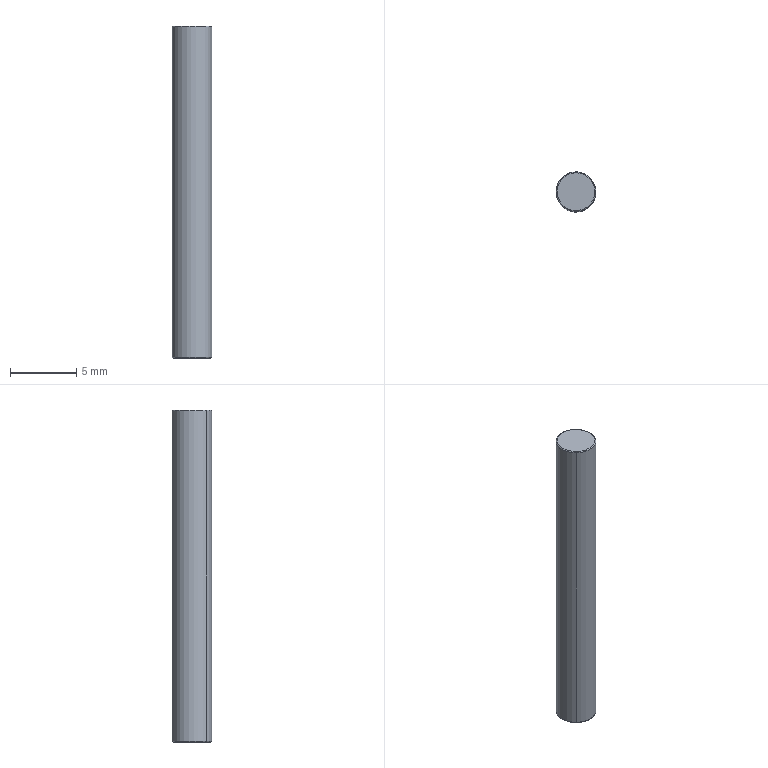Part | SolidWorks | features SplitBody 1 | 1 solid | 8 faces | box 3 x 3 x 25 mm | volume 176.692 mm3 | torus 4 | cylinder 2 | plane 2 | commonest cylinder face diameters 3 x2
STEP:
#1=CARTESIAN_POINT('',(423.091,-5.089,-249.647));
#2=VERTEX_POINT('',#1);
#3=CARTESIAN_POINT('',(425.059,-3.028,-249.647));
#4=VERTEX_POINT('',#3);
#5=CARTESIAN_POINT('',(424.075,-4.058,-249.647));
#6=DIRECTION('',(0.,0.,1.));
#7=DIRECTION('',(0.6906,0.7232,0.));
#8=AXIS2_PLACEMENT_3D('',#5,#6,#7);
#9=CIRCLE('',#8,1.425);
#10=EDGE_CURVE('',#2,#4,#9,.T.);
#11=ORIENTED_EDGE('',*,*,#10,.F.);
#12=CARTESIAN_POINT('',(423.039,-5.143,-249.722));
#13=VERTEX_POINT('',#12);
#14=CARTESIAN_POINT('',(423.091,-5.089,-249.722));
#15=DIRECTION('',(0.7232,-0.6906,0.));
#16=DIRECTION('',(0.6906,0.7232,0.));
#17=AXIS2_PLACEMENT_3D('',#14,#15,#16);
#18=CIRCLE('',#17,0.075);
#19=EDGE_CURVE('',#2,#13,#18,.T.);
#20=ORIENTED_EDGE('',*,*,#19,.T.);
#21=CARTESIAN_POINT('',(425.111,-2.974,-249.722));
#22=VERTEX_POINT('',#21);
#23=CARTESIAN_POINT('',(424.075,-4.058,-249.722));
#24=DIRECTION('',(0.,0.,-1.));
#25=DIRECTION('',(0.6906,0.7232,0.));
#26=AXIS2_PLACEMENT_3D('',#23,#24,#25);
#27=CIRCLE('',#26,1.5);
#28=EDGE_CURVE('',#22,#13,#27,.T.);
#29=ORIENTED_EDGE('',*,*,#28,.F.);
#30=CARTESIAN_POINT('',(425.059,-3.028,-249.722));
#31=DIRECTION('',(-0.7232,0.6906,0.));
#32=DIRECTION('',(-0.6906,-0.7232,0.));
#33=AXIS2_PLACEMENT_3D('',#30,#31,#32);
#34=CIRCLE('',#33,0.075);
#35=EDGE_CURVE('',#4,#22,#34,.T.);
#36=ORIENTED_EDGE('',*,*,#35,.F.);
#37=EDGE_LOOP('',(#11,#20,#29,#36));
#38=FACE_OUTER_BOUND('',#37,.T.);
#39=CARTESIAN_POINT('',(424.075,-4.058,-249.722));
#40=DIRECTION('',(0.,0.,-1.));
#41=DIRECTION('',(0.6906,0.7232,0.));
#42=AXIS2_PLACEMENT_3D('',#39,#40,#41);
#43=TOROIDAL_SURFACE('',#42,1.425,0.075);
#44=ADVANCED_FACE('',(#38),#43,.T.);
#45=CARTESIAN_POINT('',(423.039,-5.143,-274.572));
#46=VERTEX_POINT('',#45);
#47=CARTESIAN_POINT('',(425.111,-2.974,-274.572));
#48=VERTEX_POINT('',#47);
#49=CARTESIAN_POINT('',(424.075,-4.058,-274.572));
#50=DIRECTION('',(0.,0.,1.));
#51=DIRECTION('',(0.6906,0.7232,0.));
#52=AXIS2_PLACEMENT_3D('',#49,#50,#51);
#53=CIRCLE('',#52,1.5);
#54=EDGE_CURVE('',#46,#48,#53,.T.);
#55=ORIENTED_EDGE('',*,*,#54,.F.);
#56=CARTESIAN_POINT('',(423.091,-5.089,-274.647));
#57=VERTEX_POINT('',#56);
#58=CARTESIAN_POINT('',(423.091,-5.089,-274.572));
#59=DIRECTION('',(0.7232,-0.6906,0.));
#60=DIRECTION('',(0.6906,0.7232,0.));
#61=AXIS2_PLACEMENT_3D('',#58,#59,#60);
#62=CIRCLE('',#61,0.075);
#63=EDGE_CURVE('',#46,#57,#62,.T.);
#64=ORIENTED_EDGE('',*,*,#63,.T.);
#65=CARTESIAN_POINT('',(425.059,-3.028,-274.647));
#66=VERTEX_POINT('',#65);
#67=CARTESIAN_POINT('',(424.075,-4.058,-274.647));
#68=DIRECTION('',(0.,0.,-1.));
#69=DIRECTION('',(0.6906,0.7232,0.));
#70=AXIS2_PLACEMENT_3D('',#67,#68,#69);
#71=CIRCLE('',#70,1.425);
#72=EDGE_CURVE('',#66,#57,#71,.T.);
#73=ORIENTED_EDGE('',*,*,#72,.F.);
#74=CARTESIAN_POINT('',(425.059,-3.028,-274.572));
#75=DIRECTION('',(-0.7232,0.6906,0.));
#76=DIRECTION('',(-0.6906,-0.7232,0.));
#77=AXIS2_PLACEMENT_3D('',#74,#75,#76);
#78=CIRCLE('',#77,0.075);
#79=EDGE_CURVE('',#48,#66,#78,.T.);
#80=ORIENTED_EDGE('',*,*,#79,.F.);
#81=EDGE_LOOP('',(#55,#64,#73,#80));
#82=FACE_OUTER_BOUND('',#81,.T.);
#83=CARTESIAN_POINT('',(424.075,-4.058,-274.572));
#84=DIRECTION('',(0.,0.,-1.));
#85=DIRECTION('',(0.6906,0.7232,0.));
#86=AXIS2_PLACEMENT_3D('',#83,#84,#85);
#87=TOROIDAL_SURFACE('',#86,1.425,0.075);
#88=ADVANCED_FACE('',(#82),#87,.T.);
#89=ORIENTED_EDGE('',*,*,#28,.T.);
#90=CARTESIAN_POINT('',(423.039,-5.143,-249.647));
#91=DIRECTION('',(0.,0.,-1.));
#92=VECTOR('',#91,1000.);
#93=LINE('',#90,#92);
#94=EDGE_CURVE('',#13,#46,#93,.T.);
#95=ORIENTED_EDGE('',*,*,#94,.T.);
#96=ORIENTED_EDGE('',*,*,#54,.T.);
#97=CARTESIAN_POINT('',(425.111,-2.974,-249.647));
#98=DIRECTION('',(0.,0.,-1.));
#99=VECTOR('',#98,1000.);
#100=LINE('',#97,#99);
#101=EDGE_CURVE('',#22,#48,#100,.T.);
#102=ORIENTED_EDGE('',*,*,#101,.F.);
#103=EDGE_LOOP('',(#89,#95,#96,#102));
#104=FACE_OUTER_BOUND('',#103,.T.);
#105=CARTESIAN_POINT('',(424.075,-4.058,-249.647));
#106=DIRECTION('',(0.,0.,-1.));
#107=DIRECTION('',(0.6906,0.7232,0.));
#108=AXIS2_PLACEMENT_3D('',#105,#106,#107);
#109=CYLINDRICAL_SURFACE('',#108,1.5);
#110=ADVANCED_FACE('',(#104),#109,.T.);
#111=ORIENTED_EDGE('',*,*,#94,.F.);
#112=CARTESIAN_POINT('',(424.075,-4.058,-249.722));
#113=DIRECTION('',(0.,0.,-1.));
#114=DIRECTION('',(0.6906,0.7232,0.));
#115=AXIS2_PLACEMENT_3D('',#112,#113,#114);
#116=CIRCLE('',#115,1.5);
#117=EDGE_CURVE('',#13,#22,#116,.T.);
#118=ORIENTED_EDGE('',*,*,#117,.T.);
#119=ORIENTED_EDGE('',*,*,#101,.T.);
#120=CARTESIAN_POINT('',(424.075,-4.058,-274.572));
#121=DIRECTION('',(0.,0.,1.));
#122=DIRECTION('',(0.6906,0.7232,0.));
#123=AXIS2_PLACEMENT_3D('',#120,#121,#122);
#124=CIRCLE('',#123,1.5);
#125=EDGE_CURVE('',#48,#46,#124,.T.);
#126=ORIENTED_EDGE('',*,*,#125,.T.);
#127=EDGE_LOOP('',(#111,#118,#119,#126));
#128=FACE_OUTER_BOUND('',#127,.T.);
#129=CARTESIAN_POINT('',(424.075,-4.058,-249.647));
#130=DIRECTION('',(0.,0.,-1.));
#131=DIRECTION('',(0.6906,0.7232,0.));
#132=AXIS2_PLACEMENT_3D('',#129,#130,#131);
#133=CYLINDRICAL_SURFACE('',#132,1.5);
#134=ADVANCED_FACE('',(#128),#133,.T.);
#135=CARTESIAN_POINT('',(424.075,-4.058,-249.647));
#136=DIRECTION('',(0.,0.,1.));
#137=DIRECTION('',(0.6906,0.7232,0.));
#138=AXIS2_PLACEMENT_3D('',#135,#136,#137);
#139=CIRCLE('',#138,1.425);
#140=EDGE_CURVE('',#4,#2,#139,.T.);
#141=ORIENTED_EDGE('',*,*,#140,.T.);
#142=ORIENTED_EDGE('',*,*,#10,.T.);
#143=EDGE_LOOP('',(#141,#142));
#144=FACE_OUTER_BOUND('',#143,.T.);
#145=CARTESIAN_POINT('',(424.075,-4.058,-249.647));
#146=DIRECTION('',(0.,0.,-1.));
#147=DIRECTION('',(0.6906,0.7232,0.));
#148=AXIS2_PLACEMENT_3D('',#145,#146,#147);
#149=PLANE('',#148);
#150=ADVANCED_FACE('',(#144),#149,.F.);
#151=ORIENTED_EDGE('',*,*,#72,.T.);
#152=CARTESIAN_POINT('',(424.075,-4.058,-274.647));
#153=DIRECTION('',(0.,0.,-1.));
#154=DIRECTION('',(0.6906,0.7232,0.));
#155=AXIS2_PLACEMENT_3D('',#152,#153,#154);
#156=CIRCLE('',#155,1.425);
#157=EDGE_CURVE('',#57,#66,#156,.T.);
#158=ORIENTED_EDGE('',*,*,#157,.T.);
#159=EDGE_LOOP('',(#151,#158));
#160=FACE_OUTER_BOUND('',#159,.T.);
#161=CARTESIAN_POINT('',(424.075,-4.058,-274.647));
#162=DIRECTION('',(0.,0.,-1.));
#163=DIRECTION('',(0.6906,0.7232,0.));
#164=AXIS2_PLACEMENT_3D('',#161,#162,#163);
#165=PLANE('',#164);
#166=ADVANCED_FACE('',(#160),#165,.T.);
#167=ORIENTED_EDGE('',*,*,#63,.F.);
#168=ORIENTED_EDGE('',*,*,#125,.F.);
#169=ORIENTED_EDGE('',*,*,#79,.T.);
#170=ORIENTED_EDGE('',*,*,#157,.F.);
#171=EDGE_LOOP('',(#167,#168,#169,#170));
#172=FACE_OUTER_BOUND('',#171,.T.);
#173=CARTESIAN_POINT('',(424.075,-4.058,-274.572));
#174=DIRECTION('',(0.,0.,-1.));
#175=DIRECTION('',(0.6906,0.7232,0.));
#176=AXIS2_PLACEMENT_3D('',#173,#174,#175);
#177=TOROIDAL_SURFACE('',#176,1.425,0.075);
#178=ADVANCED_FACE('',(#172),#177,.T.);
#179=ORIENTED_EDGE('',*,*,#19,.F.);
#180=ORIENTED_EDGE('',*,*,#140,.F.);
#181=ORIENTED_EDGE('',*,*,#35,.T.);
#182=ORIENTED_EDGE('',*,*,#117,.F.);
#183=EDGE_LOOP('',(#179,#180,#181,#182));
#184=FACE_OUTER_BOUND('',#183,.T.);
#185=CARTESIAN_POINT('',(424.075,-4.058,-249.722));
#186=DIRECTION('',(0.,0.,-1.));
#187=DIRECTION('',(0.6906,0.7232,0.));
#188=AXIS2_PLACEMENT_3D('',#185,#186,#187);
#189=TOROIDAL_SURFACE('',#188,1.425,0.075);
#190=ADVANCED_FACE('',(#184),#189,.T.);
#191=CLOSED_SHELL('',(#44,#88,#110,#134,#150,#166,#178,#190));
#192=MANIFOLD_SOLID_BREP('',#191);
#193=CARTESIAN_POINT('',(0.,0.,0.));
#194=DIRECTION('',(0.,0.,1.));
#195=DIRECTION('',(1.,0.,0.));
#196=AXIS2_PLACEMENT_3D('',#193,#194,#195);
#197=(LENGTH_UNIT()NAMED_UNIT(*)SI_UNIT(.MILLI.,.METRE.));
#198=UNCERTAINTY_MEASURE_WITH_UNIT(LENGTH_MEASURE(0.00001),#197,'','');
#199=(NAMED_UNIT(*)PLANE_ANGLE_UNIT()SI_UNIT($,.RADIAN.));
#200=(NAMED_UNIT(*)SI_UNIT($,.STERADIAN.)SOLID_ANGLE_UNIT());
#201=(GEOMETRIC_REPRESENTATION_CONTEXT(3)GLOBAL_UNCERTAINTY_ASSIGNED_CONTEXT((#198))GLOBAL_UNIT_ASSIGNED_CONTEXT((#197,#199,#200))REPRESENTATION_CONTEXT('',''));
#202=ADVANCED_BREP_SHAPE_REPRESENTATION('',(#192,#196),#201);